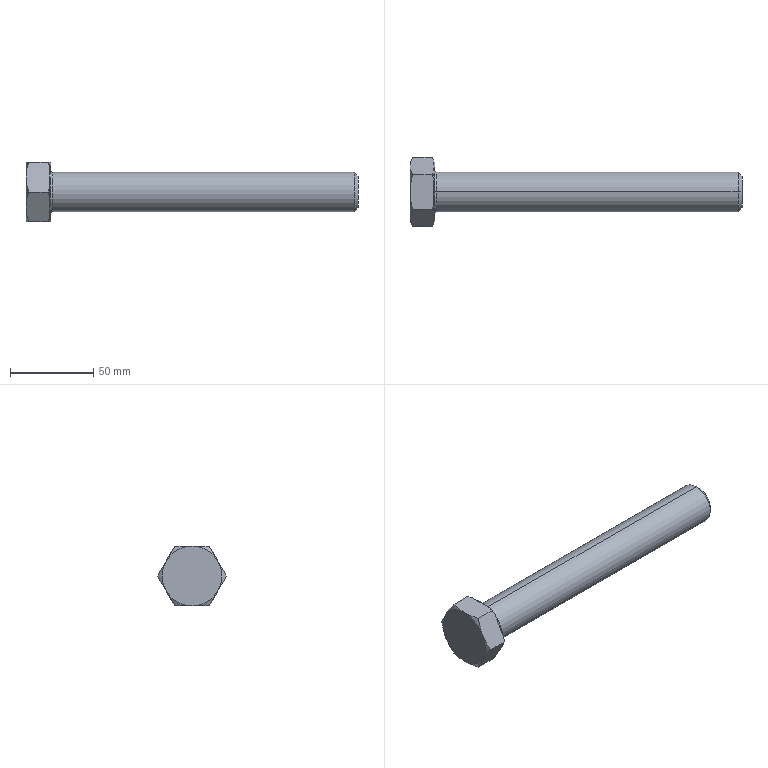Part | SolidWorks | features RevCut 4, Chamfer 1, Extrusion 1, Fillet 1, LPattern 1, Revolution 1 | 1 solid | 35 faces | box 200 x 41.569 x 36 mm | volume 100195 mm3 | plane 15 | cone 14 | cylinder 4 | torus 2 | commonest cylinder face diameters 24 x2 36 x2
STEP:
#1=CARTESIAN_POINT('',(15.8,0.,12.));
#2=VERTEX_POINT('',#1);
#3=CARTESIAN_POINT('',(15.8,0.,-12.));
#4=VERTEX_POINT('',#3);
#5=CARTESIAN_POINT('',(15.8,0.,0.));
#6=DIRECTION('',(1.,0.,0.));
#7=DIRECTION('',(0.,0.,-1.));
#8=AXIS2_PLACEMENT_3D('',#5,#6,#7);
#9=CIRCLE('',#8,12.);
#10=EDGE_CURVE('',#2,#4,#9,.T.);
#11=ORIENTED_EDGE('',*,*,#10,.F.);
#12=CARTESIAN_POINT('',(15.,0.,12.8));
#13=VERTEX_POINT('',#12);
#14=CARTESIAN_POINT('',(15.8,0.,12.8));
#15=DIRECTION('',(0.,1.,0.));
#16=DIRECTION('',(0.,0.,1.));
#17=AXIS2_PLACEMENT_3D('',#14,#15,#16);
#18=CIRCLE('',#17,0.8);
#19=EDGE_CURVE('',#2,#13,#18,.T.);
#20=ORIENTED_EDGE('',*,*,#19,.T.);
#21=CARTESIAN_POINT('',(15.,0.,-12.8));
#22=VERTEX_POINT('',#21);
#23=CARTESIAN_POINT('',(15.,0.,0.));
#24=DIRECTION('',(-1.,0.,0.));
#25=DIRECTION('',(0.,0.,-1.));
#26=AXIS2_PLACEMENT_3D('',#23,#24,#25);
#27=CIRCLE('',#26,12.8);
#28=EDGE_CURVE('',#22,#13,#27,.T.);
#29=ORIENTED_EDGE('',*,*,#28,.F.);
#30=CARTESIAN_POINT('',(15.8,0.,-12.8));
#31=DIRECTION('',(0.,-1.,0.));
#32=DIRECTION('',(0.,0.,-1.));
#33=AXIS2_PLACEMENT_3D('',#30,#31,#32);
#34=CIRCLE('',#33,0.8);
#35=EDGE_CURVE('',#4,#22,#34,.T.);
#36=ORIENTED_EDGE('',*,*,#35,.F.);
#37=EDGE_LOOP('',(#11,#20,#29,#36));
#38=FACE_OUTER_BOUND('',#37,.T.);
#39=CARTESIAN_POINT('',(15.8,0.,0.));
#40=DIRECTION('',(1.,0.,0.));
#41=DIRECTION('',(0.,0.,-1.));
#42=AXIS2_PLACEMENT_3D('',#39,#40,#41);
#43=TOROIDAL_SURFACE('',#42,12.8,0.8);
#44=ADVANCED_FACE('',(#38),#43,.F.);
#45=CARTESIAN_POINT('',(200.,0.,-9.6));
#46=VERTEX_POINT('',#45);
#47=CARTESIAN_POINT('',(200.,0.,9.6));
#48=VERTEX_POINT('',#47);
#49=CARTESIAN_POINT('',(200.,0.,0.));
#50=DIRECTION('',(1.,0.,0.));
#51=DIRECTION('',(0.,0.,1.));
#52=AXIS2_PLACEMENT_3D('',#49,#50,#51);
#53=CIRCLE('',#52,9.6);
#54=EDGE_CURVE('',#46,#48,#53,.T.);
#55=ORIENTED_EDGE('',*,*,#54,.F.);
#56=CARTESIAN_POINT('',(197.6,0.,-12.));
#57=VERTEX_POINT('',#56);
#58=CARTESIAN_POINT('',(197.6,0.,-12.));
#59=DIRECTION('',(-0.7071,0.,-0.7071));
#60=VECTOR('',#59,1000.);
#61=LINE('',#58,#60);
#62=EDGE_CURVE('',#46,#57,#61,.T.);
#63=ORIENTED_EDGE('',*,*,#62,.T.);
#64=CARTESIAN_POINT('',(197.6,0.,12.));
#65=VERTEX_POINT('',#64);
#66=CARTESIAN_POINT('',(197.6,0.,0.));
#67=DIRECTION('',(-1.,0.,0.));
#68=DIRECTION('',(0.,0.,1.));
#69=AXIS2_PLACEMENT_3D('',#66,#67,#68);
#70=CIRCLE('',#69,12.);
#71=EDGE_CURVE('',#65,#57,#70,.T.);
#72=ORIENTED_EDGE('',*,*,#71,.F.);
#73=CARTESIAN_POINT('',(197.6,0.,12.));
#74=DIRECTION('',(-0.7071,0.,0.7071));
#75=VECTOR('',#74,1000.);
#76=LINE('',#73,#75);
#77=EDGE_CURVE('',#48,#65,#76,.T.);
#78=ORIENTED_EDGE('',*,*,#77,.F.);
#79=EDGE_LOOP('',(#55,#63,#72,#78));
#80=FACE_OUTER_BOUND('',#79,.T.);
#81=CARTESIAN_POINT('',(197.6,0.,0.));
#82=DIRECTION('',(-1.,0.,0.));
#83=DIRECTION('',(0.,0.,1.));
#84=AXIS2_PLACEMENT_3D('',#81,#82,#83);
#85=CONICAL_SURFACE('',#84,12.,0.7854);
#86=ADVANCED_FACE('',(#80),#85,.T.);
#87=ORIENTED_EDGE('',*,*,#71,.T.);
#88=CARTESIAN_POINT('',(0.,0.,-12.));
#89=DIRECTION('',(-1.,0.,0.));
#90=VECTOR('',#89,1000.);
#91=LINE('',#88,#90);
#92=EDGE_CURVE('',#57,#4,#91,.T.);
#93=ORIENTED_EDGE('',*,*,#92,.T.);
#94=CARTESIAN_POINT('',(15.8,0.,0.));
#95=DIRECTION('',(1.,0.,0.));
#96=DIRECTION('',(0.,0.,-1.));
#97=AXIS2_PLACEMENT_3D('',#94,#95,#96);
#98=CIRCLE('',#97,12.);
#99=EDGE_CURVE('',#4,#2,#98,.T.);
#100=ORIENTED_EDGE('',*,*,#99,.T.);
#101=CARTESIAN_POINT('',(0.,0.,12.));
#102=DIRECTION('',(-1.,0.,0.));
#103=VECTOR('',#102,1000.);
#104=LINE('',#101,#103);
#105=EDGE_CURVE('',#65,#2,#104,.T.);
#106=ORIENTED_EDGE('',*,*,#105,.F.);
#107=EDGE_LOOP('',(#87,#93,#100,#106));
#108=FACE_OUTER_BOUND('',#107,.T.);
#109=CARTESIAN_POINT('',(0.,0.,0.));
#110=DIRECTION('',(-1.,0.,0.));
#111=DIRECTION('',(0.,0.,1.));
#112=AXIS2_PLACEMENT_3D('',#109,#110,#111);
#113=CYLINDRICAL_SURFACE('',#112,12.);
#114=ADVANCED_FACE('',(#108),#113,.T.);
#115=CARTESIAN_POINT('',(15.,0.,-18.));
#116=VERTEX_POINT('',#115);
#117=CARTESIAN_POINT('',(15.,0.,18.));
#118=VERTEX_POINT('',#117);
#119=CARTESIAN_POINT('',(15.,0.,0.));
#120=DIRECTION('',(1.,0.,0.));
#121=DIRECTION('',(0.,0.,-1.));
#122=AXIS2_PLACEMENT_3D('',#119,#120,#121);
#123=CIRCLE('',#122,18.);
#124=EDGE_CURVE('',#116,#118,#123,.T.);
#125=ORIENTED_EDGE('',*,*,#124,.F.);
#126=CARTESIAN_POINT('',(14.2,0.,-18.));
#127=VERTEX_POINT('',#126);
#128=CARTESIAN_POINT('',(0.,0.,-18.));
#129=DIRECTION('',(-1.,0.,0.));
#130=VECTOR('',#129,1000.);
#131=LINE('',#128,#130);
#132=EDGE_CURVE('',#116,#127,#131,.T.);
#133=ORIENTED_EDGE('',*,*,#132,.T.);
#134=CARTESIAN_POINT('',(14.2,15.588,-9.));
#135=VERTEX_POINT('',#134);
#136=CARTESIAN_POINT('',(14.2,0.,0.));
#137=DIRECTION('',(-1.,0.,0.));
#138=DIRECTION('',(0.,0.,1.));
#139=AXIS2_PLACEMENT_3D('',#136,#137,#138);
#140=CIRCLE('',#139,18.);
#141=EDGE_CURVE('',#135,#127,#140,.T.);
#142=ORIENTED_EDGE('',*,*,#141,.F.);
#143=CARTESIAN_POINT('',(14.2,15.588,9.));
#144=VERTEX_POINT('',#143);
#145=CARTESIAN_POINT('',(14.2,0.,0.));
#146=DIRECTION('',(-1.,0.,0.));
#147=DIRECTION('',(0.,0.,1.));
#148=AXIS2_PLACEMENT_3D('',#145,#146,#147);
#149=CIRCLE('',#148,18.);
#150=EDGE_CURVE('',#144,#135,#149,.T.);
#151=ORIENTED_EDGE('',*,*,#150,.F.);
#152=CARTESIAN_POINT('',(14.2,0.,18.));
#153=VERTEX_POINT('',#152);
#154=CARTESIAN_POINT('',(14.2,0.,0.));
#155=DIRECTION('',(-1.,0.,0.));
#156=DIRECTION('',(0.,0.,1.));
#157=AXIS2_PLACEMENT_3D('',#154,#155,#156);
#158=CIRCLE('',#157,18.);
#159=EDGE_CURVE('',#153,#144,#158,.T.);
#160=ORIENTED_EDGE('',*,*,#159,.F.);
#161=CARTESIAN_POINT('',(0.,0.,18.));
#162=DIRECTION('',(-1.,0.,0.));
#163=VECTOR('',#162,1000.);
#164=LINE('',#161,#163);
#165=EDGE_CURVE('',#118,#153,#164,.T.);
#166=ORIENTED_EDGE('',*,*,#165,.F.);
#167=EDGE_LOOP('',(#125,#133,#142,#151,#160,#166));
#168=FACE_OUTER_BOUND('',#167,.T.);
#169=CARTESIAN_POINT('',(0.,0.,0.));
#170=DIRECTION('',(-1.,0.,0.));
#171=DIRECTION('',(0.,0.,1.));
#172=AXIS2_PLACEMENT_3D('',#169,#170,#171);
#173=CYLINDRICAL_SURFACE('',#172,18.);
#174=ADVANCED_FACE('',(#168),#173,.T.);
#175=CARTESIAN_POINT('',(14.2,11.99,-15.233));
#176=VERTEX_POINT('',#175);
#177=CARTESIAN_POINT('',(14.2,10.392,-18.));
#178=DIRECTION('',(0.,0.5,0.866));
#179=VECTOR('',#178,1000.);
#180=LINE('',#177,#179);
#181=EDGE_CURVE('',#176,#135,#180,.T.);
#182=ORIENTED_EDGE('',*,*,#181,.F.);
#183=CARTESIAN_POINT('',(13.392,10.392,-18.));
#184=VERTEX_POINT('',#183);
#185=CARTESIAN_POINT('',(13.392,10.392,-18.));
#186=CARTESIAN_POINT('',(13.698,10.922,-17.082));
#187=CARTESIAN_POINT('',(13.97,11.454,-16.16));
#188=CARTESIAN_POINT('',(14.2,11.99,-15.233));
#189=B_SPLINE_CURVE_WITH_KNOTS('',3,(#185,#186,#187,#188),.UNSPECIFIED.,.F.,.F.,(4,4),(0.000000238,0.003277),.UNSPECIFIED.);
#190=EDGE_CURVE('',#184,#176,#189,.T.);
#191=ORIENTED_EDGE('',*,*,#190,.F.);
#192=CARTESIAN_POINT('',(1.608,10.392,-18.));
#193=VERTEX_POINT('',#192);
#194=CARTESIAN_POINT('',(15.,10.392,-18.));
#195=DIRECTION('',(-1.,0.,0.));
#196=VECTOR('',#195,1000.);
#197=LINE('',#194,#196);
#198=EDGE_CURVE('',#184,#193,#197,.T.);
#199=ORIENTED_EDGE('',*,*,#198,.T.);
#200=CARTESIAN_POINT('',(0.,15.588,-9.));
#201=VERTEX_POINT('',#200);
#202=CARTESIAN_POINT('',(0.,15.588,-9.));
#203=CARTESIAN_POINT('',(0.,15.368,-9.382));
#204=CARTESIAN_POINT('',(0.009429,15.146,-9.766));
#205=CARTESIAN_POINT('',(0.04683,14.705,-10.53));
#206=CARTESIAN_POINT('',(0.07476,14.485,-10.91));
#207=CARTESIAN_POINT('',(0.1851,13.828,-12.049));
#208=CARTESIAN_POINT('',(0.294,13.393,-12.803));
#209=CARTESIAN_POINT('',(0.714,12.095,-15.051));
#210=CARTESIAN_POINT('',(1.118,11.24,-16.531));
#211=CARTESIAN_POINT('',(1.608,10.392,-18.));
#212=B_SPLINE_CURVE_WITH_KNOTS('',3,(#202,#203,#204,#205,#206,#207,#208,#209,#210,#211),.UNSPECIFIED.,.F.,.F.,(4,2,2,2,4),(0.01052,0.01183,0.01313,0.01575,0.02099),.UNSPECIFIED.);
#213=EDGE_CURVE('',#201,#193,#212,.T.);
#214=ORIENTED_EDGE('',*,*,#213,.F.);
#215=CARTESIAN_POINT('',(1.608,20.785,0.));
#216=VERTEX_POINT('',#215);
#217=CARTESIAN_POINT('',(1.608,20.785,0.));
#218=CARTESIAN_POINT('',(1.117,19.935,-1.472));
#219=CARTESIAN_POINT('',(0.7126,19.078,-2.955));
#220=CARTESIAN_POINT('',(0.1532,17.348,-5.952));
#221=CARTESIAN_POINT('',(0.,16.474,-7.467));
#222=CARTESIAN_POINT('',(0.,15.588,-9.));
#223=B_SPLINE_CURVE_WITH_KNOTS('',3,(#217,#218,#219,#220,#221,#222),.UNSPECIFIED.,.F.,.F.,(4,2,4),(0.000000238,0.005258,0.01052),.UNSPECIFIED.);
#224=EDGE_CURVE('',#216,#201,#223,.T.);
#225=ORIENTED_EDGE('',*,*,#224,.F.);
#226=CARTESIAN_POINT('',(13.392,20.785,0.));
#227=VERTEX_POINT('',#226);
#228=CARTESIAN_POINT('',(15.,20.785,0.));
#229=DIRECTION('',(-1.,0.,0.));
#230=VECTOR('',#229,1000.);
#231=LINE('',#228,#230);
#232=EDGE_CURVE('',#227,#216,#231,.T.);
#233=ORIENTED_EDGE('',*,*,#232,.F.);
#234=CARTESIAN_POINT('',(14.2,19.187,-2.767));
#235=VERTEX_POINT('',#234);
#236=CARTESIAN_POINT('',(14.2,19.187,-2.767));
#237=CARTESIAN_POINT('',(13.97,19.723,-1.839));
#238=CARTESIAN_POINT('',(13.698,20.255,-0.9171));
#239=CARTESIAN_POINT('',(13.392,20.785,0.));
#240=B_SPLINE_CURVE_WITH_KNOTS('',3,(#236,#237,#238,#239),.UNSPECIFIED.,.F.,.F.,(4,4),(0.01772,0.02099),.UNSPECIFIED.);
#241=EDGE_CURVE('',#235,#227,#240,.T.);
#242=ORIENTED_EDGE('',*,*,#241,.F.);
#243=CARTESIAN_POINT('',(14.2,10.392,-18.));
#244=DIRECTION('',(0.,0.5,0.866));
#245=VECTOR('',#244,1000.);
#246=LINE('',#243,#245);
#247=EDGE_CURVE('',#135,#235,#246,.T.);
#248=ORIENTED_EDGE('',*,*,#247,.F.);
#249=EDGE_LOOP('',(#182,#191,#199,#214,#225,#233,#242,#248));
#250=FACE_OUTER_BOUND('',#249,.T.);
#251=CARTESIAN_POINT('',(15.,10.392,-18.));
#252=DIRECTION('',(0.,-0.866,0.5));
#253=DIRECTION('',(0.,-0.5,-0.866));
#254=AXIS2_PLACEMENT_3D('',#251,#252,#253);
#255=PLANE('',#254);
#256=ADVANCED_FACE('',(#250),#255,.F.);
#257=CARTESIAN_POINT('',(14.2,19.187,2.767));
#258=VERTEX_POINT('',#257);
#259=CARTESIAN_POINT('',(14.2,20.785,0.));
#260=DIRECTION('',(0.,-0.5,0.866));
#261=VECTOR('',#260,1000.);
#262=LINE('',#259,#261);
#263=EDGE_CURVE('',#258,#144,#262,.T.);
#264=ORIENTED_EDGE('',*,*,#263,.F.);
#265=CARTESIAN_POINT('',(13.392,20.785,0.));
#266=CARTESIAN_POINT('',(13.698,20.255,0.9177));
#267=CARTESIAN_POINT('',(13.97,19.723,1.84));
#268=CARTESIAN_POINT('',(14.2,19.187,2.767));
#269=B_SPLINE_CURVE_WITH_KNOTS('',3,(#265,#266,#267,#268),.UNSPECIFIED.,.F.,.F.,(4,4),(0.000000238,0.003277),.UNSPECIFIED.);
#270=EDGE_CURVE('',#227,#258,#269,.T.);
#271=ORIENTED_EDGE('',*,*,#270,.F.);
#272=ORIENTED_EDGE('',*,*,#232,.T.);
#273=CARTESIAN_POINT('',(0.,15.588,9.));
#274=VERTEX_POINT('',#273);
#275=CARTESIAN_POINT('',(0.,15.588,9.));
#276=CARTESIAN_POINT('',(0.,15.809,8.618));
#277=CARTESIAN_POINT('',(0.009429,16.031,8.234));
#278=CARTESIAN_POINT('',(0.04683,16.472,7.47));
#279=CARTESIAN_POINT('',(0.07476,16.691,7.09));
#280=CARTESIAN_POINT('',(0.1851,17.349,5.951));
#281=CARTESIAN_POINT('',(0.294,17.784,5.197));
#282=CARTESIAN_POINT('',(0.714,19.082,2.949));
#283=CARTESIAN_POINT('',(1.118,19.937,1.469));
#284=CARTESIAN_POINT('',(1.608,20.785,0.));
#285=B_SPLINE_CURVE_WITH_KNOTS('',3,(#275,#276,#277,#278,#279,#280,#281,#282,#283,#284),.UNSPECIFIED.,.F.,.F.,(4,2,2,2,4),(0.01052,0.01183,0.01313,0.01575,0.02099),.UNSPECIFIED.);
#286=EDGE_CURVE('',#274,#216,#285,.T.);
#287=ORIENTED_EDGE('',*,*,#286,.F.);
#288=CARTESIAN_POINT('',(1.608,10.392,18.));
#289=VERTEX_POINT('',#288);
#290=CARTESIAN_POINT('',(1.608,10.392,18.));
#291=CARTESIAN_POINT('',(1.117,11.242,16.528));
#292=CARTESIAN_POINT('',(0.7126,12.099,15.045));
#293=CARTESIAN_POINT('',(0.1532,13.829,12.048));
#294=CARTESIAN_POINT('',(0.,14.703,10.533));
#295=CARTESIAN_POINT('',(0.,15.588,9.));
#296=B_SPLINE_CURVE_WITH_KNOTS('',3,(#290,#291,#292,#293,#294,#295),.UNSPECIFIED.,.F.,.F.,(4,2,4),(0.000000238,0.005258,0.01052),.UNSPECIFIED.);
#297=EDGE_CURVE('',#289,#274,#296,.T.);
#298=ORIENTED_EDGE('',*,*,#297,.F.);
#299=CARTESIAN_POINT('',(13.392,10.392,18.));
#300=VERTEX_POINT('',#299);
#301=CARTESIAN_POINT('',(15.,10.392,18.));
#302=DIRECTION('',(-1.,0.,0.));
#303=VECTOR('',#302,1000.);
#304=LINE('',#301,#303);
#305=EDGE_CURVE('',#300,#289,#304,.T.);
#306=ORIENTED_EDGE('',*,*,#305,.F.);
#307=CARTESIAN_POINT('',(14.2,11.99,15.233));
#308=VERTEX_POINT('',#307);
#309=CARTESIAN_POINT('',(14.2,11.99,15.233));
#310=CARTESIAN_POINT('',(13.97,11.454,16.161));
#311=CARTESIAN_POINT('',(13.698,10.922,17.083));
#312=CARTESIAN_POINT('',(13.392,10.392,18.));
#313=B_SPLINE_CURVE_WITH_KNOTS('',3,(#309,#310,#311,#312),.UNSPECIFIED.,.F.,.F.,(4,4),(0.01772,0.02099),.UNSPECIFIED.);
#314=EDGE_CURVE('',#308,#300,#313,.T.);
#315=ORIENTED_EDGE('',*,*,#314,.F.);
#316=CARTESIAN_POINT('',(14.2,20.785,0.));
#317=DIRECTION('',(0.,-0.5,0.866));
#318=VECTOR('',#317,1000.);
#319=LINE('',#316,#318);
#320=EDGE_CURVE('',#144,#308,#319,.T.);
#321=ORIENTED_EDGE('',*,*,#320,.F.);
#322=EDGE_LOOP('',(#264,#271,#272,#287,#298,#306,#315,#321));
#323=FACE_OUTER_BOUND('',#322,.T.);
#324=CARTESIAN_POINT('',(15.,20.785,0.));
#325=DIRECTION('',(0.,-0.866,-0.5));
#326=DIRECTION('',(0.,0.5,-0.866));
#327=AXIS2_PLACEMENT_3D('',#324,#325,#326);
#328=PLANE('',#327);
#329=ADVANCED_FACE('',(#323),#328,.F.);
#330=CARTESIAN_POINT('',(14.2,7.197,18.));
#331=VERTEX_POINT('',#330);
#332=CARTESIAN_POINT('',(14.2,10.392,18.));
#333=DIRECTION('',(0.,-1.,0.));
#334=VECTOR('',#333,1000.);
#335=LINE('',#332,#334);
#336=EDGE_CURVE('',#331,#153,#335,.T.);
#337=ORIENTED_EDGE('',*,*,#336,.F.);
#338=CARTESIAN_POINT('',(13.392,10.392,18.));
#339=CARTESIAN_POINT('',(13.697,9.337,18.));
#340=CARTESIAN_POINT('',(13.97,8.273,18.));
#341=CARTESIAN_POINT('',(14.2,7.197,18.));
#342=B_SPLINE_CURVE_WITH_KNOTS('',3,(#338,#339,#340,#341),.UNSPECIFIED.,.F.,.F.,(4,4),(0.04709,0.0504),.UNSPECIFIED.);
#343=EDGE_CURVE('',#300,#331,#342,.T.);
#344=ORIENTED_EDGE('',*,*,#343,.F.);
#345=ORIENTED_EDGE('',*,*,#305,.T.);
#346=CARTESIAN_POINT('',(0.,0.,18.));
#347=VERTEX_POINT('',#346);
#348=CARTESIAN_POINT('',(0.,0.,18.));
#349=CARTESIAN_POINT('',(0.,0.8793,18.));
#350=CARTESIAN_POINT('',(0.03746,1.762,18.));
#351=CARTESIAN_POINT('',(0.1861,3.532,18.));
#352=CARTESIAN_POINT('',(0.2962,4.408,18.));
#353=CARTESIAN_POINT('',(0.7187,7.009,18.));
#354=CARTESIAN_POINT('',(1.123,8.712,18.));
#355=CARTESIAN_POINT('',(1.608,10.392,18.));
#356=B_SPLINE_CURVE_WITH_KNOTS('',3,(#348,#349,#350,#351,#352,#353,#354,#355),.UNSPECIFIED.,.F.,.F.,(4,2,2,4),(0.02951,0.03214,0.03477,0.04003),.UNSPECIFIED.);
#357=EDGE_CURVE('',#347,#289,#356,.T.);
#358=ORIENTED_EDGE('',*,*,#357,.F.);
#359=CARTESIAN_POINT('',(1.608,-10.392,18.));
#360=VERTEX_POINT('',#359);
#361=CARTESIAN_POINT('',(1.608,-10.392,18.));
#362=CARTESIAN_POINT('',(1.364,-9.547,18.));
#363=CARTESIAN_POINT('',(1.139,-8.692,18.));
#364=CARTESIAN_POINT('',(0.742,-6.968,18.));
#365=CARTESIAN_POINT('',(0.5706,-6.103,18.));
#366=CARTESIAN_POINT('',(0.1511,-3.502,18.));
#367=CARTESIAN_POINT('',(0.,-1.757,18.));
#368=CARTESIAN_POINT('',(0.,0.,18.));
#369=B_SPLINE_CURVE_WITH_KNOTS('',3,(#361,#362,#363,#364,#365,#366,#367,#368),.UNSPECIFIED.,.F.,.F.,(4,2,2,4),(0.01899,0.02162,0.02425,0.02951),.UNSPECIFIED.);
#370=EDGE_CURVE('',#360,#347,#369,.T.);
#371=ORIENTED_EDGE('',*,*,#370,.F.);
#372=CARTESIAN_POINT('',(13.392,-10.392,18.));
#373=VERTEX_POINT('',#372);
#374=CARTESIAN_POINT('',(15.,-10.392,18.));
#375=DIRECTION('',(-1.,0.,0.));
#376=VECTOR('',#375,1000.);
#377=LINE('',#374,#376);
#378=EDGE_CURVE('',#373,#360,#377,.T.);
#379=ORIENTED_EDGE('',*,*,#378,.F.);
#380=CARTESIAN_POINT('',(14.2,-7.197,18.));
#381=VERTEX_POINT('',#380);
#382=CARTESIAN_POINT('',(14.2,-7.197,18.));
#383=CARTESIAN_POINT('',(14.085,-7.734,18.));
#384=CARTESIAN_POINT('',(13.959,-8.271,18.));
#385=CARTESIAN_POINT('',(13.688,-9.337,18.));
#386=CARTESIAN_POINT('',(13.544,-9.866,18.));
#387=CARTESIAN_POINT('',(13.392,-10.392,18.));
#388=B_SPLINE_CURVE_WITH_KNOTS('',3,(#382,#383,#384,#385,#386,#387),.UNSPECIFIED.,.F.,.F.,(4,2,4),(0.06487,0.06651,0.06814),.UNSPECIFIED.);
#389=EDGE_CURVE('',#381,#373,#388,.T.);
#390=ORIENTED_EDGE('',*,*,#389,.F.);
#391=CARTESIAN_POINT('',(14.2,10.392,18.));
#392=DIRECTION('',(0.,-1.,0.));
#393=VECTOR('',#392,1000.);
#394=LINE('',#391,#393);
#395=EDGE_CURVE('',#153,#381,#394,.T.);
#396=ORIENTED_EDGE('',*,*,#395,.F.);
#397=EDGE_LOOP('',(#337,#344,#345,#358,#371,#379,#390,#396));
#398=FACE_OUTER_BOUND('',#397,.T.);
#399=CARTESIAN_POINT('',(15.,10.392,18.));
#400=DIRECTION('',(0.,0.,-1.));
#401=DIRECTION('',(-1.,0.,0.));
#402=AXIS2_PLACEMENT_3D('',#399,#400,#401);
#403=PLANE('',#402);
#404=ADVANCED_FACE('',(#398),#403,.F.);
#405=CARTESIAN_POINT('',(14.2,-11.99,15.233));
#406=VERTEX_POINT('',#405);
#407=CARTESIAN_POINT('',(14.2,-15.588,9.));
#408=VERTEX_POINT('',#407);
#409=CARTESIAN_POINT('',(14.2,-20.785,0.));
#410=DIRECTION('',(0.,-0.5,-0.866));
#411=VECTOR('',#410,1000.);
#412=LINE('',#409,#411);
#413=EDGE_CURVE('',#406,#408,#412,.T.);
#414=ORIENTED_EDGE('',*,*,#413,.F.);
#415=CARTESIAN_POINT('',(13.392,-10.392,18.));
#416=CARTESIAN_POINT('',(13.698,-10.922,17.082));
#417=CARTESIAN_POINT('',(13.97,-11.454,16.16));
#418=CARTESIAN_POINT('',(14.2,-11.99,15.233));
#419=B_SPLINE_CURVE_WITH_KNOTS('',3,(#415,#416,#417,#418),.UNSPECIFIED.,.F.,.F.,(4,4),(0.000000238,0.003277),.UNSPECIFIED.);
#420=EDGE_CURVE('',#373,#406,#419,.T.);
#421=ORIENTED_EDGE('',*,*,#420,.F.);
#422=ORIENTED_EDGE('',*,*,#378,.T.);
#423=CARTESIAN_POINT('',(0.,-15.588,9.));
#424=VERTEX_POINT('',#423);
#425=CARTESIAN_POINT('',(0.,-15.588,9.));
#426=CARTESIAN_POINT('',(0.,-15.368,9.382));
#427=CARTESIAN_POINT('',(0.009429,-15.146,9.766));
#428=CARTESIAN_POINT('',(0.04683,-14.705,10.53));
#429=CARTESIAN_POINT('',(0.07476,-14.485,10.91));
#430=CARTESIAN_POINT('',(0.1851,-13.828,12.049));
#431=CARTESIAN_POINT('',(0.294,-13.393,12.803));
#432=CARTESIAN_POINT('',(0.714,-12.095,15.051));
#433=CARTESIAN_POINT('',(1.118,-11.24,16.531));
#434=CARTESIAN_POINT('',(1.608,-10.392,18.));
#435=B_SPLINE_CURVE_WITH_KNOTS('',3,(#425,#426,#427,#428,#429,#430,#431,#432,#433,#434),.UNSPECIFIED.,.F.,.F.,(4,2,2,2,4),(0.01052,0.01183,0.01313,0.01575,0.02099),.UNSPECIFIED.);
#436=EDGE_CURVE('',#424,#360,#435,.T.);
#437=ORIENTED_EDGE('',*,*,#436,.F.);
#438=CARTESIAN_POINT('',(1.608,-20.785,0.));
#439=VERTEX_POINT('',#438);
#440=CARTESIAN_POINT('',(1.608,-20.785,0.));
#441=CARTESIAN_POINT('',(1.117,-19.935,1.472));
#442=CARTESIAN_POINT('',(0.7126,-19.078,2.955));
#443=CARTESIAN_POINT('',(0.1532,-17.348,5.952));
#444=CARTESIAN_POINT('',(0.,-16.474,7.467));
#445=CARTESIAN_POINT('',(0.,-15.588,9.));
#446=B_SPLINE_CURVE_WITH_KNOTS('',3,(#440,#441,#442,#443,#444,#445),.UNSPECIFIED.,.F.,.F.,(4,2,4),(0.000000238,0.005258,0.01052),.UNSPECIFIED.);
#447=EDGE_CURVE('',#439,#424,#446,.T.);
#448=ORIENTED_EDGE('',*,*,#447,.F.);
#449=CARTESIAN_POINT('',(13.392,-20.785,0.));
#450=VERTEX_POINT('',#449);
#451=CARTESIAN_POINT('',(15.,-20.785,0.));
#452=DIRECTION('',(-1.,0.,0.));
#453=VECTOR('',#452,1000.);
#454=LINE('',#451,#453);
#455=EDGE_CURVE('',#450,#439,#454,.T.);
#456=ORIENTED_EDGE('',*,*,#455,.F.);
#457=CARTESIAN_POINT('',(14.2,-19.187,2.767));
#458=VERTEX_POINT('',#457);
#459=CARTESIAN_POINT('',(14.2,-19.187,2.767));
#460=CARTESIAN_POINT('',(13.97,-19.723,1.839));
#461=CARTESIAN_POINT('',(13.698,-20.255,0.9171));
#462=CARTESIAN_POINT('',(13.392,-20.785,0.));
#463=B_SPLINE_CURVE_WITH_KNOTS('',3,(#459,#460,#461,#462),.UNSPECIFIED.,.F.,.F.,(4,4),(0.01772,0.02099),.UNSPECIFIED.);
#464=EDGE_CURVE('',#458,#450,#463,.T.);
#465=ORIENTED_EDGE('',*,*,#464,.F.);
#466=CARTESIAN_POINT('',(14.2,-20.785,0.));
#467=DIRECTION('',(0.,-0.5,-0.866));
#468=VECTOR('',#467,1000.);
#469=LINE('',#466,#468);
#470=EDGE_CURVE('',#408,#458,#469,.T.);
#471=ORIENTED_EDGE('',*,*,#470,.F.);
#472=EDGE_LOOP('',(#414,#421,#422,#437,#448,#456,#465,#471));
#473=FACE_OUTER_BOUND('',#472,.T.);
#474=CARTESIAN_POINT('',(15.,-20.785,0.));
#475=DIRECTION('',(0.,0.866,-0.5));
#476=DIRECTION('',(0.,0.5,0.866));
#477=AXIS2_PLACEMENT_3D('',#474,#475,#476);
#478=PLANE('',#477);
#479=ADVANCED_FACE('',(#473),#478,.F.);
#480=CARTESIAN_POINT('',(14.2,-19.187,-2.767));
#481=VERTEX_POINT('',#480);
#482=CARTESIAN_POINT('',(14.2,-15.588,-9.));
#483=VERTEX_POINT('',#482);
#484=CARTESIAN_POINT('',(14.2,-10.392,-18.));
#485=DIRECTION('',(0.,0.5,-0.866));
#486=VECTOR('',#485,1000.);
#487=LINE('',#484,#486);
#488=EDGE_CURVE('',#481,#483,#487,.T.);
#489=ORIENTED_EDGE('',*,*,#488,.F.);
#490=CARTESIAN_POINT('',(13.392,-20.785,0.));
#491=CARTESIAN_POINT('',(13.698,-20.255,-0.9177));
#492=CARTESIAN_POINT('',(13.97,-19.723,-1.84));
#493=CARTESIAN_POINT('',(14.2,-19.187,-2.767));
#494=B_SPLINE_CURVE_WITH_KNOTS('',3,(#490,#491,#492,#493),.UNSPECIFIED.,.F.,.F.,(4,4),(0.000000238,0.003277),.UNSPECIFIED.);
#495=EDGE_CURVE('',#450,#481,#494,.T.);
#496=ORIENTED_EDGE('',*,*,#495,.F.);
#497=ORIENTED_EDGE('',*,*,#455,.T.);
#498=CARTESIAN_POINT('',(0.,-15.588,-9.));
#499=VERTEX_POINT('',#498);
#500=CARTESIAN_POINT('',(0.,-15.588,-9.));
#501=CARTESIAN_POINT('',(0.,-15.809,-8.618));
#502=CARTESIAN_POINT('',(0.009429,-16.031,-8.234));
#503=CARTESIAN_POINT('',(0.04683,-16.472,-7.47));
#504=CARTESIAN_POINT('',(0.07476,-16.691,-7.09));
#505=CARTESIAN_POINT('',(0.1851,-17.349,-5.951));
#506=CARTESIAN_POINT('',(0.294,-17.784,-5.197));
#507=CARTESIAN_POINT('',(0.714,-19.082,-2.949));
#508=CARTESIAN_POINT('',(1.118,-19.937,-1.469));
#509=CARTESIAN_POINT('',(1.608,-20.785,0.));
#510=B_SPLINE_CURVE_WITH_KNOTS('',3,(#500,#501,#502,#503,#504,#505,#506,#507,#508,#509),.UNSPECIFIED.,.F.,.F.,(4,2,2,2,4),(0.01052,0.01183,0.01313,0.01575,0.02099),.UNSPECIFIED.);
#511=EDGE_CURVE('',#499,#439,#510,.T.);
#512=ORIENTED_EDGE('',*,*,#511,.F.);
#513=CARTESIAN_POINT('',(1.608,-10.392,-18.));
#514=VERTEX_POINT('',#513);
#515=CARTESIAN_POINT('',(1.608,-10.392,-18.));
#516=CARTESIAN_POINT('',(1.117,-11.242,-16.528));
#517=CARTESIAN_POINT('',(0.7126,-12.099,-15.045));
#518=CARTESIAN_POINT('',(0.1532,-13.829,-12.048));
#519=CARTESIAN_POINT('',(0.,-14.703,-10.533));
#520=CARTESIAN_POINT('',(0.,-15.588,-9.));
#521=B_SPLINE_CURVE_WITH_KNOTS('',3,(#515,#516,#517,#518,#519,#520),.UNSPECIFIED.,.F.,.F.,(4,2,4),(0.000000238,0.005258,0.01052),.UNSPECIFIED.);
#522=EDGE_CURVE('',#514,#499,#521,.T.);
#523=ORIENTED_EDGE('',*,*,#522,.F.);
#524=CARTESIAN_POINT('',(13.392,-10.392,-18.));
#525=VERTEX_POINT('',#524);
#526=CARTESIAN_POINT('',(15.,-10.392,-18.));
#527=DIRECTION('',(-1.,0.,0.));
#528=VECTOR('',#527,1000.);
#529=LINE('',#526,#528);
#530=EDGE_CURVE('',#525,#514,#529,.T.);
#531=ORIENTED_EDGE('',*,*,#530,.F.);
#532=CARTESIAN_POINT('',(14.2,-11.99,-15.233));
#533=VERTEX_POINT('',#532);
#534=CARTESIAN_POINT('',(14.2,-11.99,-15.233));
#535=CARTESIAN_POINT('',(13.97,-11.454,-16.161));
#536=CARTESIAN_POINT('',(13.698,-10.922,-17.083));
#537=CARTESIAN_POINT('',(13.392,-10.392,-18.));
#538=B_SPLINE_CURVE_WITH_KNOTS('',3,(#534,#535,#536,#537),.UNSPECIFIED.,.F.,.F.,(4,4),(0.01772,0.02099),.UNSPECIFIED.);
#539=EDGE_CURVE('',#533,#525,#538,.T.);
#540=ORIENTED_EDGE('',*,*,#539,.F.);
#541=CARTESIAN_POINT('',(14.2,-10.392,-18.));
#542=DIRECTION('',(0.,0.5,-0.866));
#543=VECTOR('',#542,1000.);
#544=LINE('',#541,#543);
#545=EDGE_CURVE('',#483,#533,#544,.T.);
#546=ORIENTED_EDGE('',*,*,#545,.F.);
#547=EDGE_LOOP('',(#489,#496,#497,#512,#523,#531,#540,#546));
#548=FACE_OUTER_BOUND('',#547,.T.);
#549=CARTESIAN_POINT('',(15.,-10.392,-18.));
#550=DIRECTION('',(0.,0.866,0.5));
#551=DIRECTION('',(0.,-0.5,0.866));
#552=AXIS2_PLACEMENT_3D('',#549,#550,#551);
#553=PLANE('',#552);
#554=ADVANCED_FACE('',(#548),#553,.F.);
#555=CARTESIAN_POINT('',(14.2,-7.197,-18.));
#556=VERTEX_POINT('',#555);
#557=CARTESIAN_POINT('',(14.2,10.392,-18.));
#558=DIRECTION('',(0.,1.,0.));
#559=VECTOR('',#558,1000.);
#560=LINE('',#557,#559);
#561=EDGE_CURVE('',#556,#127,#560,.T.);
#562=ORIENTED_EDGE('',*,*,#561,.F.);
#563=CARTESIAN_POINT('',(13.392,-10.392,-18.));
#564=CARTESIAN_POINT('',(13.544,-9.866,-18.));
#565=CARTESIAN_POINT('',(13.688,-9.337,-18.));
#566=CARTESIAN_POINT('',(13.959,-8.271,-18.));
#567=CARTESIAN_POINT('',(14.085,-7.734,-18.));
#568=CARTESIAN_POINT('',(14.2,-7.197,-18.));
#569=B_SPLINE_CURVE_WITH_KNOTS('',3,(#563,#564,#565,#566,#567,#568),.UNSPECIFIED.,.F.,.F.,(4,2,4),(0.01899,0.02062,0.02226),.UNSPECIFIED.);
#570=EDGE_CURVE('',#525,#556,#569,.T.);
#571=ORIENTED_EDGE('',*,*,#570,.F.);
#572=ORIENTED_EDGE('',*,*,#530,.T.);
#573=CARTESIAN_POINT('',(0.,0.,-18.));
#574=VERTEX_POINT('',#573);
#575=CARTESIAN_POINT('',(0.,0.,-18.));
#576=CARTESIAN_POINT('',(0.,-1.757,-18.));
#577=CARTESIAN_POINT('',(0.1511,-3.502,-18.));
#578=CARTESIAN_POINT('',(0.5706,-6.103,-18.));
#579=CARTESIAN_POINT('',(0.742,-6.968,-18.));
#580=CARTESIAN_POINT('',(1.139,-8.692,-18.));
#581=CARTESIAN_POINT('',(1.364,-9.547,-18.));
#582=CARTESIAN_POINT('',(1.608,-10.392,-18.));
#583=B_SPLINE_CURVE_WITH_KNOTS('',3,(#575,#576,#577,#578,#579,#580,#581,#582),.UNSPECIFIED.,.F.,.F.,(4,2,2,4),(0.05762,0.06288,0.06551,0.06814),.UNSPECIFIED.);
#584=EDGE_CURVE('',#574,#514,#583,.T.);
#585=ORIENTED_EDGE('',*,*,#584,.F.);
#586=CARTESIAN_POINT('',(1.608,10.392,-18.));
#587=CARTESIAN_POINT('',(1.123,8.712,-18.));
#588=CARTESIAN_POINT('',(0.7187,7.009,-18.));
#589=CARTESIAN_POINT('',(0.2962,4.408,-18.));
#590=CARTESIAN_POINT('',(0.1861,3.532,-18.));
#591=CARTESIAN_POINT('',(0.03746,1.762,-18.));
#592=CARTESIAN_POINT('',(0.,0.8793,-18.));
#593=CARTESIAN_POINT('',(0.,0.,-18.));
#594=B_SPLINE_CURVE_WITH_KNOTS('',3,(#586,#587,#588,#589,#590,#591,#592,#593),.UNSPECIFIED.,.F.,.F.,(4,2,2,4),(0.04709,0.05235,0.05499,0.05762),.UNSPECIFIED.);
#595=EDGE_CURVE('',#193,#574,#594,.T.);
#596=ORIENTED_EDGE('',*,*,#595,.F.);
#597=ORIENTED_EDGE('',*,*,#198,.F.);
#598=CARTESIAN_POINT('',(14.2,7.197,-18.));
#599=VERTEX_POINT('',#598);
#600=CARTESIAN_POINT('',(14.2,7.197,-18.));
#601=CARTESIAN_POINT('',(13.97,8.273,-18.));
#602=CARTESIAN_POINT('',(13.697,9.337,-18.));
#603=CARTESIAN_POINT('',(13.392,10.392,-18.));
#604=B_SPLINE_CURVE_WITH_KNOTS('',3,(#600,#601,#602,#603),.UNSPECIFIED.,.F.,.F.,(4,4),(0.03673,0.04003),.UNSPECIFIED.);
#605=EDGE_CURVE('',#599,#184,#604,.T.);
#606=ORIENTED_EDGE('',*,*,#605,.F.);
#607=CARTESIAN_POINT('',(14.2,10.392,-18.));
#608=DIRECTION('',(0.,1.,0.));
#609=VECTOR('',#608,1000.);
#610=LINE('',#607,#609);
#611=EDGE_CURVE('',#127,#599,#610,.T.);
#612=ORIENTED_EDGE('',*,*,#611,.F.);
#613=EDGE_LOOP('',(#562,#571,#572,#585,#596,#597,#606,#612));
#614=FACE_OUTER_BOUND('',#613,.T.);
#615=CARTESIAN_POINT('',(15.,10.392,-18.));
#616=DIRECTION('',(0.,0.,1.));
#617=DIRECTION('',(0.,-1.,0.));
#618=AXIS2_PLACEMENT_3D('',#615,#616,#617);
#619=PLANE('',#618);
#620=ADVANCED_FACE('',(#614),#619,.F.);
#621=ORIENTED_EDGE('',*,*,#570,.T.);
#622=CARTESIAN_POINT('',(14.2,0.,0.));
#623=DIRECTION('',(-1.,0.,0.));
#624=DIRECTION('',(0.,0.,-1.));
#625=AXIS2_PLACEMENT_3D('',#622,#623,#624);
#626=CIRCLE('',#625,19.386);
#627=EDGE_CURVE('',#556,#533,#626,.T.);
#628=ORIENTED_EDGE('',*,*,#627,.T.);
#629=ORIENTED_EDGE('',*,*,#539,.T.);
#630=EDGE_LOOP('',(#621,#628,#629));
#631=FACE_OUTER_BOUND('',#630,.T.);
#632=CARTESIAN_POINT('',(10.506,0.,0.));
#633=DIRECTION('',(-1.,0.,0.));
#634=DIRECTION('',(0.,0.,1.));
#635=AXIS2_PLACEMENT_3D('',#632,#633,#634);
#636=CONICAL_SURFACE('',#635,25.785,1.047);
#637=ADVANCED_FACE('',(#631),#636,.T.);
#638=ORIENTED_EDGE('',*,*,#495,.T.);
#639=CARTESIAN_POINT('',(14.2,0.,0.));
#640=DIRECTION('',(-1.,0.,0.));
#641=DIRECTION('',(0.,0.,-1.));
#642=AXIS2_PLACEMENT_3D('',#639,#640,#641);
#643=CIRCLE('',#642,19.386);
#644=EDGE_CURVE('',#481,#458,#643,.T.);
#645=ORIENTED_EDGE('',*,*,#644,.T.);
#646=ORIENTED_EDGE('',*,*,#464,.T.);
#647=EDGE_LOOP('',(#638,#645,#646));
#648=FACE_OUTER_BOUND('',#647,.T.);
#649=CARTESIAN_POINT('',(10.506,0.,0.));
#650=DIRECTION('',(-1.,0.,0.));
#651=DIRECTION('',(0.,0.,1.));
#652=AXIS2_PLACEMENT_3D('',#649,#650,#651);
#653=CONICAL_SURFACE('',#652,25.785,1.047);
#654=ADVANCED_FACE('',(#648),#653,.T.);
#655=ORIENTED_EDGE('',*,*,#420,.T.);
#656=CARTESIAN_POINT('',(14.2,0.,0.));
#657=DIRECTION('',(-1.,0.,0.));
#658=DIRECTION('',(0.,0.,-1.));
#659=AXIS2_PLACEMENT_3D('',#656,#657,#658);
#660=CIRCLE('',#659,19.386);
#661=EDGE_CURVE('',#406,#381,#660,.T.);
#662=ORIENTED_EDGE('',*,*,#661,.T.);
#663=ORIENTED_EDGE('',*,*,#389,.T.);
#664=EDGE_LOOP('',(#655,#662,#663));
#665=FACE_OUTER_BOUND('',#664,.T.);
#666=CARTESIAN_POINT('',(10.506,0.,0.));
#667=DIRECTION('',(-1.,0.,0.));
#668=DIRECTION('',(0.,0.,1.));
#669=AXIS2_PLACEMENT_3D('',#666,#667,#668);
#670=CONICAL_SURFACE('',#669,25.785,1.047);
#671=ADVANCED_FACE('',(#665),#670,.T.);
#672=ORIENTED_EDGE('',*,*,#343,.T.);
#673=CARTESIAN_POINT('',(14.2,0.,0.));
#674=DIRECTION('',(-1.,0.,0.));
#675=DIRECTION('',(0.,0.,-1.));
#676=AXIS2_PLACEMENT_3D('',#673,#674,#675);
#677=CIRCLE('',#676,19.386);
#678=EDGE_CURVE('',#331,#308,#677,.T.);
#679=ORIENTED_EDGE('',*,*,#678,.T.);
#680=ORIENTED_EDGE('',*,*,#314,.T.);
#681=EDGE_LOOP('',(#672,#679,#680));
#682=FACE_OUTER_BOUND('',#681,.T.);
#683=CARTESIAN_POINT('',(10.506,0.,0.));
#684=DIRECTION('',(-1.,0.,0.));
#685=DIRECTION('',(0.,0.,1.));
#686=AXIS2_PLACEMENT_3D('',#683,#684,#685);
#687=CONICAL_SURFACE('',#686,25.785,1.047);
#688=ADVANCED_FACE('',(#682),#687,.T.);
#689=ORIENTED_EDGE('',*,*,#270,.T.);
#690=CARTESIAN_POINT('',(14.2,0.,0.));
#691=DIRECTION('',(-1.,0.,0.));
#692=DIRECTION('',(0.,0.,-1.));
#693=AXIS2_PLACEMENT_3D('',#690,#691,#692);
#694=CIRCLE('',#693,19.386);
#695=EDGE_CURVE('',#258,#235,#694,.T.);
#696=ORIENTED_EDGE('',*,*,#695,.T.);
#697=ORIENTED_EDGE('',*,*,#241,.T.);
#698=EDGE_LOOP('',(#689,#696,#697));
#699=FACE_OUTER_BOUND('',#698,.T.);
#700=CARTESIAN_POINT('',(10.506,0.,0.));
#701=DIRECTION('',(-1.,0.,0.));
#702=DIRECTION('',(0.,0.,1.));
#703=AXIS2_PLACEMENT_3D('',#700,#701,#702);
#704=CONICAL_SURFACE('',#703,25.785,1.047);
#705=ADVANCED_FACE('',(#699),#704,.T.);
#706=ORIENTED_EDGE('',*,*,#190,.T.);
#707=CARTESIAN_POINT('',(14.2,0.,0.));
#708=DIRECTION('',(-1.,0.,0.));
#709=DIRECTION('',(0.,0.,-1.));
#710=AXIS2_PLACEMENT_3D('',#707,#708,#709);
#711=CIRCLE('',#710,19.386);
#712=EDGE_CURVE('',#176,#599,#711,.T.);
#713=ORIENTED_EDGE('',*,*,#712,.T.);
#714=ORIENTED_EDGE('',*,*,#605,.T.);
#715=EDGE_LOOP('',(#706,#713,#714));
#716=FACE_OUTER_BOUND('',#715,.T.);
#717=CARTESIAN_POINT('',(10.506,0.,0.));
#718=DIRECTION('',(-1.,0.,0.));
#719=DIRECTION('',(0.,0.,1.));
#720=AXIS2_PLACEMENT_3D('',#717,#718,#719);
#721=CONICAL_SURFACE('',#720,25.785,1.047);
#722=ADVANCED_FACE('',(#716),#721,.T.);
#723=ORIENTED_EDGE('',*,*,#522,.T.);
#724=CARTESIAN_POINT('',(0.,0.,0.));
#725=DIRECTION('',(1.,0.,0.));
#726=DIRECTION('',(0.,0.,-1.));
#727=AXIS2_PLACEMENT_3D('',#724,#725,#726);
#728=CIRCLE('',#727,18.);
#729=EDGE_CURVE('',#499,#574,#728,.T.);
#730=ORIENTED_EDGE('',*,*,#729,.T.);
#731=ORIENTED_EDGE('',*,*,#584,.T.);
#732=EDGE_LOOP('',(#723,#730,#731));
#733=FACE_OUTER_BOUND('',#732,.T.);
#734=CARTESIAN_POINT('',(0.,0.,0.));
#735=DIRECTION('',(1.,0.,0.));
#736=DIRECTION('',(0.,0.,-1.));
#737=AXIS2_PLACEMENT_3D('',#734,#735,#736);
#738=CONICAL_SURFACE('',#737,18.,1.047);
#739=ADVANCED_FACE('',(#733),#738,.T.);
#740=ORIENTED_EDGE('',*,*,#447,.T.);
#741=CARTESIAN_POINT('',(0.,0.,0.));
#742=DIRECTION('',(1.,0.,0.));
#743=DIRECTION('',(0.,0.,-1.));
#744=AXIS2_PLACEMENT_3D('',#741,#742,#743);
#745=CIRCLE('',#744,18.);
#746=EDGE_CURVE('',#424,#499,#745,.T.);
#747=ORIENTED_EDGE('',*,*,#746,.T.);
#748=ORIENTED_EDGE('',*,*,#511,.T.);
#749=EDGE_LOOP('',(#740,#747,#748));
#750=FACE_OUTER_BOUND('',#749,.T.);
#751=CARTESIAN_POINT('',(0.,0.,0.));
#752=DIRECTION('',(1.,0.,0.));
#753=DIRECTION('',(0.,0.,-1.));
#754=AXIS2_PLACEMENT_3D('',#751,#752,#753);
#755=CONICAL_SURFACE('',#754,18.,1.047);
#756=ADVANCED_FACE('',(#750),#755,.T.);
#757=ORIENTED_EDGE('',*,*,#370,.T.);
#758=CARTESIAN_POINT('',(0.,0.,0.));
#759=DIRECTION('',(1.,0.,0.));
#760=DIRECTION('',(0.,0.,-1.));
#761=AXIS2_PLACEMENT_3D('',#758,#759,#760);
#762=CIRCLE('',#761,18.);
#763=EDGE_CURVE('',#347,#424,#762,.T.);
#764=ORIENTED_EDGE('',*,*,#763,.T.);
#765=ORIENTED_EDGE('',*,*,#436,.T.);
#766=EDGE_LOOP('',(#757,#764,#765));
#767=FACE_OUTER_BOUND('',#766,.T.);
#768=CARTESIAN_POINT('',(0.,0.,0.));
#769=DIRECTION('',(1.,0.,0.));
#770=DIRECTION('',(0.,0.,-1.));
#771=AXIS2_PLACEMENT_3D('',#768,#769,#770);
#772=CONICAL_SURFACE('',#771,18.,1.047);
#773=ADVANCED_FACE('',(#767),#772,.T.);
#774=ORIENTED_EDGE('',*,*,#357,.T.);
#775=ORIENTED_EDGE('',*,*,#297,.T.);
#776=CARTESIAN_POINT('',(0.,0.,0.));
#777=DIRECTION('',(-1.,0.,0.));
#778=DIRECTION('',(0.,0.,1.));
#779=AXIS2_PLACEMENT_3D('',#776,#777,#778);
#780=CIRCLE('',#779,18.);
#781=EDGE_CURVE('',#347,#274,#780,.T.);
#782=ORIENTED_EDGE('',*,*,#781,.F.);
#783=EDGE_LOOP('',(#774,#775,#782));
#784=FACE_OUTER_BOUND('',#783,.T.);
#785=CARTESIAN_POINT('',(0.,0.,0.));
#786=DIRECTION('',(1.,0.,0.));
#787=DIRECTION('',(0.,0.,-1.));
#788=AXIS2_PLACEMENT_3D('',#785,#786,#787);
#789=CONICAL_SURFACE('',#788,18.,1.047);
#790=ADVANCED_FACE('',(#784),#789,.T.);
#791=ORIENTED_EDGE('',*,*,#286,.T.);
#792=ORIENTED_EDGE('',*,*,#224,.T.);
#793=CARTESIAN_POINT('',(0.,0.,0.));
#794=DIRECTION('',(1.,0.,0.));
#795=DIRECTION('',(0.,0.,-1.));
#796=AXIS2_PLACEMENT_3D('',#793,#794,#795);
#797=CIRCLE('',#796,18.);
#798=EDGE_CURVE('',#201,#274,#797,.T.);
#799=ORIENTED_EDGE('',*,*,#798,.T.);
#800=EDGE_LOOP('',(#791,#792,#799));
#801=FACE_OUTER_BOUND('',#800,.T.);
#802=CARTESIAN_POINT('',(0.,0.,0.));
#803=DIRECTION('',(1.,0.,0.));
#804=DIRECTION('',(0.,0.,-1.));
#805=AXIS2_PLACEMENT_3D('',#802,#803,#804);
#806=CONICAL_SURFACE('',#805,18.,1.047);
#807=ADVANCED_FACE('',(#801),#806,.T.);
#808=ORIENTED_EDGE('',*,*,#213,.T.);
#809=ORIENTED_EDGE('',*,*,#595,.T.);
#810=CARTESIAN_POINT('',(0.,0.,0.));
#811=DIRECTION('',(1.,0.,0.));
#812=DIRECTION('',(0.,0.,-1.));
#813=AXIS2_PLACEMENT_3D('',#810,#811,#812);
#814=CIRCLE('',#813,18.);
#815=EDGE_CURVE('',#574,#201,#814,.T.);
#816=ORIENTED_EDGE('',*,*,#815,.T.);
#817=EDGE_LOOP('',(#808,#809,#816));
#818=FACE_OUTER_BOUND('',#817,.T.);
#819=CARTESIAN_POINT('',(0.,0.,0.));
#820=DIRECTION('',(1.,0.,0.));
#821=DIRECTION('',(0.,0.,-1.));
#822=AXIS2_PLACEMENT_3D('',#819,#820,#821);
#823=CONICAL_SURFACE('',#822,18.,1.047);
#824=ADVANCED_FACE('',(#818),#823,.T.);
#825=ORIENTED_EDGE('',*,*,#815,.F.);
#826=ORIENTED_EDGE('',*,*,#729,.F.);
#827=ORIENTED_EDGE('',*,*,#746,.F.);
#828=ORIENTED_EDGE('',*,*,#763,.F.);
#829=ORIENTED_EDGE('',*,*,#781,.T.);
#830=ORIENTED_EDGE('',*,*,#798,.F.);
#831=EDGE_LOOP('',(#825,#826,#827,#828,#829,#830));
#832=FACE_OUTER_BOUND('',#831,.T.);
#833=CARTESIAN_POINT('',(0.,20.785,0.));
#834=DIRECTION('',(1.,0.,0.));
#835=DIRECTION('',(0.,0.,-1.));
#836=AXIS2_PLACEMENT_3D('',#833,#834,#835);
#837=PLANE('',#836);
#838=ADVANCED_FACE('',(#832),#837,.F.);
#839=ORIENTED_EDGE('',*,*,#395,.T.);
#840=ORIENTED_EDGE('',*,*,#661,.F.);
#841=ORIENTED_EDGE('',*,*,#413,.T.);
#842=CARTESIAN_POINT('',(14.2,0.,0.));
#843=DIRECTION('',(-1.,0.,0.));
#844=DIRECTION('',(0.,0.,1.));
#845=AXIS2_PLACEMENT_3D('',#842,#843,#844);
#846=CIRCLE('',#845,18.);
#847=EDGE_CURVE('',#408,#153,#846,.T.);
#848=ORIENTED_EDGE('',*,*,#847,.T.);
#849=EDGE_LOOP('',(#839,#840,#841,#848));
#850=FACE_OUTER_BOUND('',#849,.T.);
#851=CARTESIAN_POINT('',(14.2,18.,0.));
#852=DIRECTION('',(1.,0.,0.));
#853=DIRECTION('',(0.,0.,-1.));
#854=AXIS2_PLACEMENT_3D('',#851,#852,#853);
#855=PLANE('',#854);
#856=ADVANCED_FACE('',(#850),#855,.T.);
#857=ORIENTED_EDGE('',*,*,#263,.T.);
#858=ORIENTED_EDGE('',*,*,#150,.T.);
#859=ORIENTED_EDGE('',*,*,#247,.T.);
#860=ORIENTED_EDGE('',*,*,#695,.F.);
#861=EDGE_LOOP('',(#857,#858,#859,#860));
#862=FACE_OUTER_BOUND('',#861,.T.);
#863=CARTESIAN_POINT('',(14.2,18.,0.));
#864=DIRECTION('',(1.,0.,0.));
#865=DIRECTION('',(0.,0.,-1.));
#866=AXIS2_PLACEMENT_3D('',#863,#864,#865);
#867=PLANE('',#866);
#868=ADVANCED_FACE('',(#862),#867,.T.);
#869=ORIENTED_EDGE('',*,*,#470,.T.);
#870=ORIENTED_EDGE('',*,*,#644,.F.);
#871=ORIENTED_EDGE('',*,*,#488,.T.);
#872=CARTESIAN_POINT('',(14.2,0.,0.));
#873=DIRECTION('',(-1.,0.,0.));
#874=DIRECTION('',(0.,0.,1.));
#875=AXIS2_PLACEMENT_3D('',#872,#873,#874);
#876=CIRCLE('',#875,18.);
#877=EDGE_CURVE('',#483,#408,#876,.T.);
#878=ORIENTED_EDGE('',*,*,#877,.T.);
#879=EDGE_LOOP('',(#869,#870,#871,#878));
#880=FACE_OUTER_BOUND('',#879,.T.);
#881=CARTESIAN_POINT('',(14.2,18.,0.));
#882=DIRECTION('',(1.,0.,0.));
#883=DIRECTION('',(0.,0.,-1.));
#884=AXIS2_PLACEMENT_3D('',#881,#882,#883);
#885=PLANE('',#884);
#886=ADVANCED_FACE('',(#880),#885,.T.);
#887=ORIENTED_EDGE('',*,*,#545,.T.);
#888=ORIENTED_EDGE('',*,*,#627,.F.);
#889=ORIENTED_EDGE('',*,*,#561,.T.);
#890=CARTESIAN_POINT('',(14.2,0.,0.));
#891=DIRECTION('',(-1.,0.,0.));
#892=DIRECTION('',(0.,0.,1.));
#893=AXIS2_PLACEMENT_3D('',#890,#891,#892);
#894=CIRCLE('',#893,18.);
#895=EDGE_CURVE('',#127,#483,#894,.T.);
#896=ORIENTED_EDGE('',*,*,#895,.T.);
#897=EDGE_LOOP('',(#887,#888,#889,#896));
#898=FACE_OUTER_BOUND('',#897,.T.);
#899=CARTESIAN_POINT('',(14.2,18.,0.));
#900=DIRECTION('',(1.,0.,0.));
#901=DIRECTION('',(0.,0.,-1.));
#902=AXIS2_PLACEMENT_3D('',#899,#900,#901);
#903=PLANE('',#902);
#904=ADVANCED_FACE('',(#898),#903,.T.);
#905=ORIENTED_EDGE('',*,*,#181,.T.);
#906=ORIENTED_EDGE('',*,*,#141,.T.);
#907=ORIENTED_EDGE('',*,*,#611,.T.);
#908=ORIENTED_EDGE('',*,*,#712,.F.);
#909=EDGE_LOOP('',(#905,#906,#907,#908));
#910=FACE_OUTER_BOUND('',#909,.T.);
#911=CARTESIAN_POINT('',(14.2,18.,0.));
#912=DIRECTION('',(1.,0.,0.));
#913=DIRECTION('',(0.,0.,-1.));
#914=AXIS2_PLACEMENT_3D('',#911,#912,#913);
#915=PLANE('',#914);
#916=ADVANCED_FACE('',(#910),#915,.T.);
#917=ORIENTED_EDGE('',*,*,#132,.F.);
#918=CARTESIAN_POINT('',(15.,0.,0.));
#919=DIRECTION('',(1.,0.,0.));
#920=DIRECTION('',(0.,0.,-1.));
#921=AXIS2_PLACEMENT_3D('',#918,#919,#920);
#922=CIRCLE('',#921,18.);
#923=EDGE_CURVE('',#118,#116,#922,.T.);
#924=ORIENTED_EDGE('',*,*,#923,.F.);
#925=ORIENTED_EDGE('',*,*,#165,.T.);
#926=ORIENTED_EDGE('',*,*,#847,.F.);
#927=ORIENTED_EDGE('',*,*,#877,.F.);
#928=ORIENTED_EDGE('',*,*,#895,.F.);
#929=EDGE_LOOP('',(#917,#924,#925,#926,#927,#928));
#930=FACE_OUTER_BOUND('',#929,.T.);
#931=CARTESIAN_POINT('',(0.,0.,0.));
#932=DIRECTION('',(-1.,0.,0.));
#933=DIRECTION('',(0.,0.,1.));
#934=AXIS2_PLACEMENT_3D('',#931,#932,#933);
#935=CYLINDRICAL_SURFACE('',#934,18.);
#936=ADVANCED_FACE('',(#930),#935,.T.);
#937=ORIENTED_EDGE('',*,*,#336,.T.);
#938=ORIENTED_EDGE('',*,*,#159,.T.);
#939=ORIENTED_EDGE('',*,*,#320,.T.);
#940=ORIENTED_EDGE('',*,*,#678,.F.);
#941=EDGE_LOOP('',(#937,#938,#939,#940));
#942=FACE_OUTER_BOUND('',#941,.T.);
#943=CARTESIAN_POINT('',(14.2,18.,0.));
#944=DIRECTION('',(1.,0.,0.));
#945=DIRECTION('',(0.,0.,-1.));
#946=AXIS2_PLACEMENT_3D('',#943,#944,#945);
#947=PLANE('',#946);
#948=ADVANCED_FACE('',(#942),#947,.T.);
#949=CARTESIAN_POINT('',(200.,0.,0.));
#950=DIRECTION('',(1.,0.,0.));
#951=DIRECTION('',(0.,0.,1.));
#952=AXIS2_PLACEMENT_3D('',#949,#950,#951);
#953=CIRCLE('',#952,9.6);
#954=EDGE_CURVE('',#48,#46,#953,.T.);
#955=ORIENTED_EDGE('',*,*,#954,.T.);
#956=ORIENTED_EDGE('',*,*,#54,.T.);
#957=EDGE_LOOP('',(#955,#956));
#958=FACE_OUTER_BOUND('',#957,.T.);
#959=CARTESIAN_POINT('',(200.,0.,0.));
#960=DIRECTION('',(-1.,0.,0.));
#961=DIRECTION('',(0.,0.,1.));
#962=AXIS2_PLACEMENT_3D('',#959,#960,#961);
#963=PLANE('',#962);
#964=ADVANCED_FACE('',(#958),#963,.F.);
#965=ORIENTED_EDGE('',*,*,#92,.F.);
#966=CARTESIAN_POINT('',(197.6,0.,0.));
#967=DIRECTION('',(-1.,0.,0.));
#968=DIRECTION('',(0.,0.,1.));
#969=AXIS2_PLACEMENT_3D('',#966,#967,#968);
#970=CIRCLE('',#969,12.);
#971=EDGE_CURVE('',#57,#65,#970,.T.);
#972=ORIENTED_EDGE('',*,*,#971,.T.);
#973=ORIENTED_EDGE('',*,*,#105,.T.);
#974=ORIENTED_EDGE('',*,*,#10,.T.);
#975=EDGE_LOOP('',(#965,#972,#973,#974));
#976=FACE_OUTER_BOUND('',#975,.T.);
#977=CARTESIAN_POINT('',(0.,0.,0.));
#978=DIRECTION('',(-1.,0.,0.));
#979=DIRECTION('',(0.,0.,1.));
#980=AXIS2_PLACEMENT_3D('',#977,#978,#979);
#981=CYLINDRICAL_SURFACE('',#980,12.);
#982=ADVANCED_FACE('',(#976),#981,.T.);
#983=ORIENTED_EDGE('',*,*,#28,.T.);
#984=CARTESIAN_POINT('',(15.,0.,0.));
#985=DIRECTION('',(-1.,0.,0.));
#986=DIRECTION('',(0.,0.,-1.));
#987=AXIS2_PLACEMENT_3D('',#984,#985,#986);
#988=CIRCLE('',#987,12.8);
#989=EDGE_CURVE('',#13,#22,#988,.T.);
#990=ORIENTED_EDGE('',*,*,#989,.T.);
#991=EDGE_LOOP('',(#983,#990));
#992=FACE_BOUND('',#991,.T.);
#993=ORIENTED_EDGE('',*,*,#923,.T.);
#994=ORIENTED_EDGE('',*,*,#124,.T.);
#995=EDGE_LOOP('',(#993,#994));
#996=FACE_OUTER_BOUND('',#995,.T.);
#997=CARTESIAN_POINT('',(15.,20.785,0.));
#998=DIRECTION('',(1.,0.,0.));
#999=DIRECTION('',(0.,0.,-1.));
#1000=AXIS2_PLACEMENT_3D('',#997,#998,#999);
#1001=PLANE('',#1000);
#1002=ADVANCED_FACE('',(#992,#996),#1001,.T.);
#1003=ORIENTED_EDGE('',*,*,#62,.F.);
#1004=ORIENTED_EDGE('',*,*,#954,.F.);
#1005=ORIENTED_EDGE('',*,*,#77,.T.);
#1006=ORIENTED_EDGE('',*,*,#971,.F.);
#1007=EDGE_LOOP('',(#1003,#1004,#1005,#1006));
#1008=FACE_OUTER_BOUND('',#1007,.T.);
#1009=CARTESIAN_POINT('',(197.6,0.,0.));
#1010=DIRECTION('',(-1.,0.,0.));
#1011=DIRECTION('',(0.,0.,1.));
#1012=AXIS2_PLACEMENT_3D('',#1009,#1010,#1011);
#1013=CONICAL_SURFACE('',#1012,12.,0.7854);
#1014=ADVANCED_FACE('',(#1008),#1013,.T.);
#1015=ORIENTED_EDGE('',*,*,#19,.F.);
#1016=ORIENTED_EDGE('',*,*,#99,.F.);
#1017=ORIENTED_EDGE('',*,*,#35,.T.);
#1018=ORIENTED_EDGE('',*,*,#989,.F.);
#1019=EDGE_LOOP('',(#1015,#1016,#1017,#1018));
#1020=FACE_OUTER_BOUND('',#1019,.T.);
#1021=CARTESIAN_POINT('',(15.8,0.,0.));
#1022=DIRECTION('',(1.,0.,0.));
#1023=DIRECTION('',(0.,0.,-1.));
#1024=AXIS2_PLACEMENT_3D('',#1021,#1022,#1023);
#1025=TOROIDAL_SURFACE('',#1024,12.8,0.8);
#1026=ADVANCED_FACE('',(#1020),#1025,.F.);
#1027=CLOSED_SHELL('',(#44,#86,#114,#174,#256,#329,#404,#479,#554,#620,#637,#654,#671,#688,#705,#722,#739,#756,#773,#790,#807,#824,#838,#856,#868,#886,#904,#916,#936,#948,#964,#982,#1002,#1014,#1026));
#1028=MANIFOLD_SOLID_BREP('',#1027);
#1029=CARTESIAN_POINT('',(0.,0.,0.));
#1030=DIRECTION('',(0.,0.,1.));
#1031=DIRECTION('',(1.,0.,0.));
#1032=AXIS2_PLACEMENT_3D('',#1029,#1030,#1031);
#1033=(LENGTH_UNIT()NAMED_UNIT(*)SI_UNIT(.MILLI.,.METRE.));
#1034=UNCERTAINTY_MEASURE_WITH_UNIT(LENGTH_MEASURE(0.00001),#1033,'','');
#1035=(NAMED_UNIT(*)PLANE_ANGLE_UNIT()SI_UNIT($,.RADIAN.));
#1036=(NAMED_UNIT(*)SI_UNIT($,.STERADIAN.)SOLID_ANGLE_UNIT());
#1037=(GEOMETRIC_REPRESENTATION_CONTEXT(3)GLOBAL_UNCERTAINTY_ASSIGNED_CONTEXT((#1034))GLOBAL_UNIT_ASSIGNED_CONTEXT((#1033,#1035,#1036))REPRESENTATION_CONTEXT('',''));
#1038=ADVANCED_BREP_SHAPE_REPRESENTATION('',(#1028,#1032),#1037);